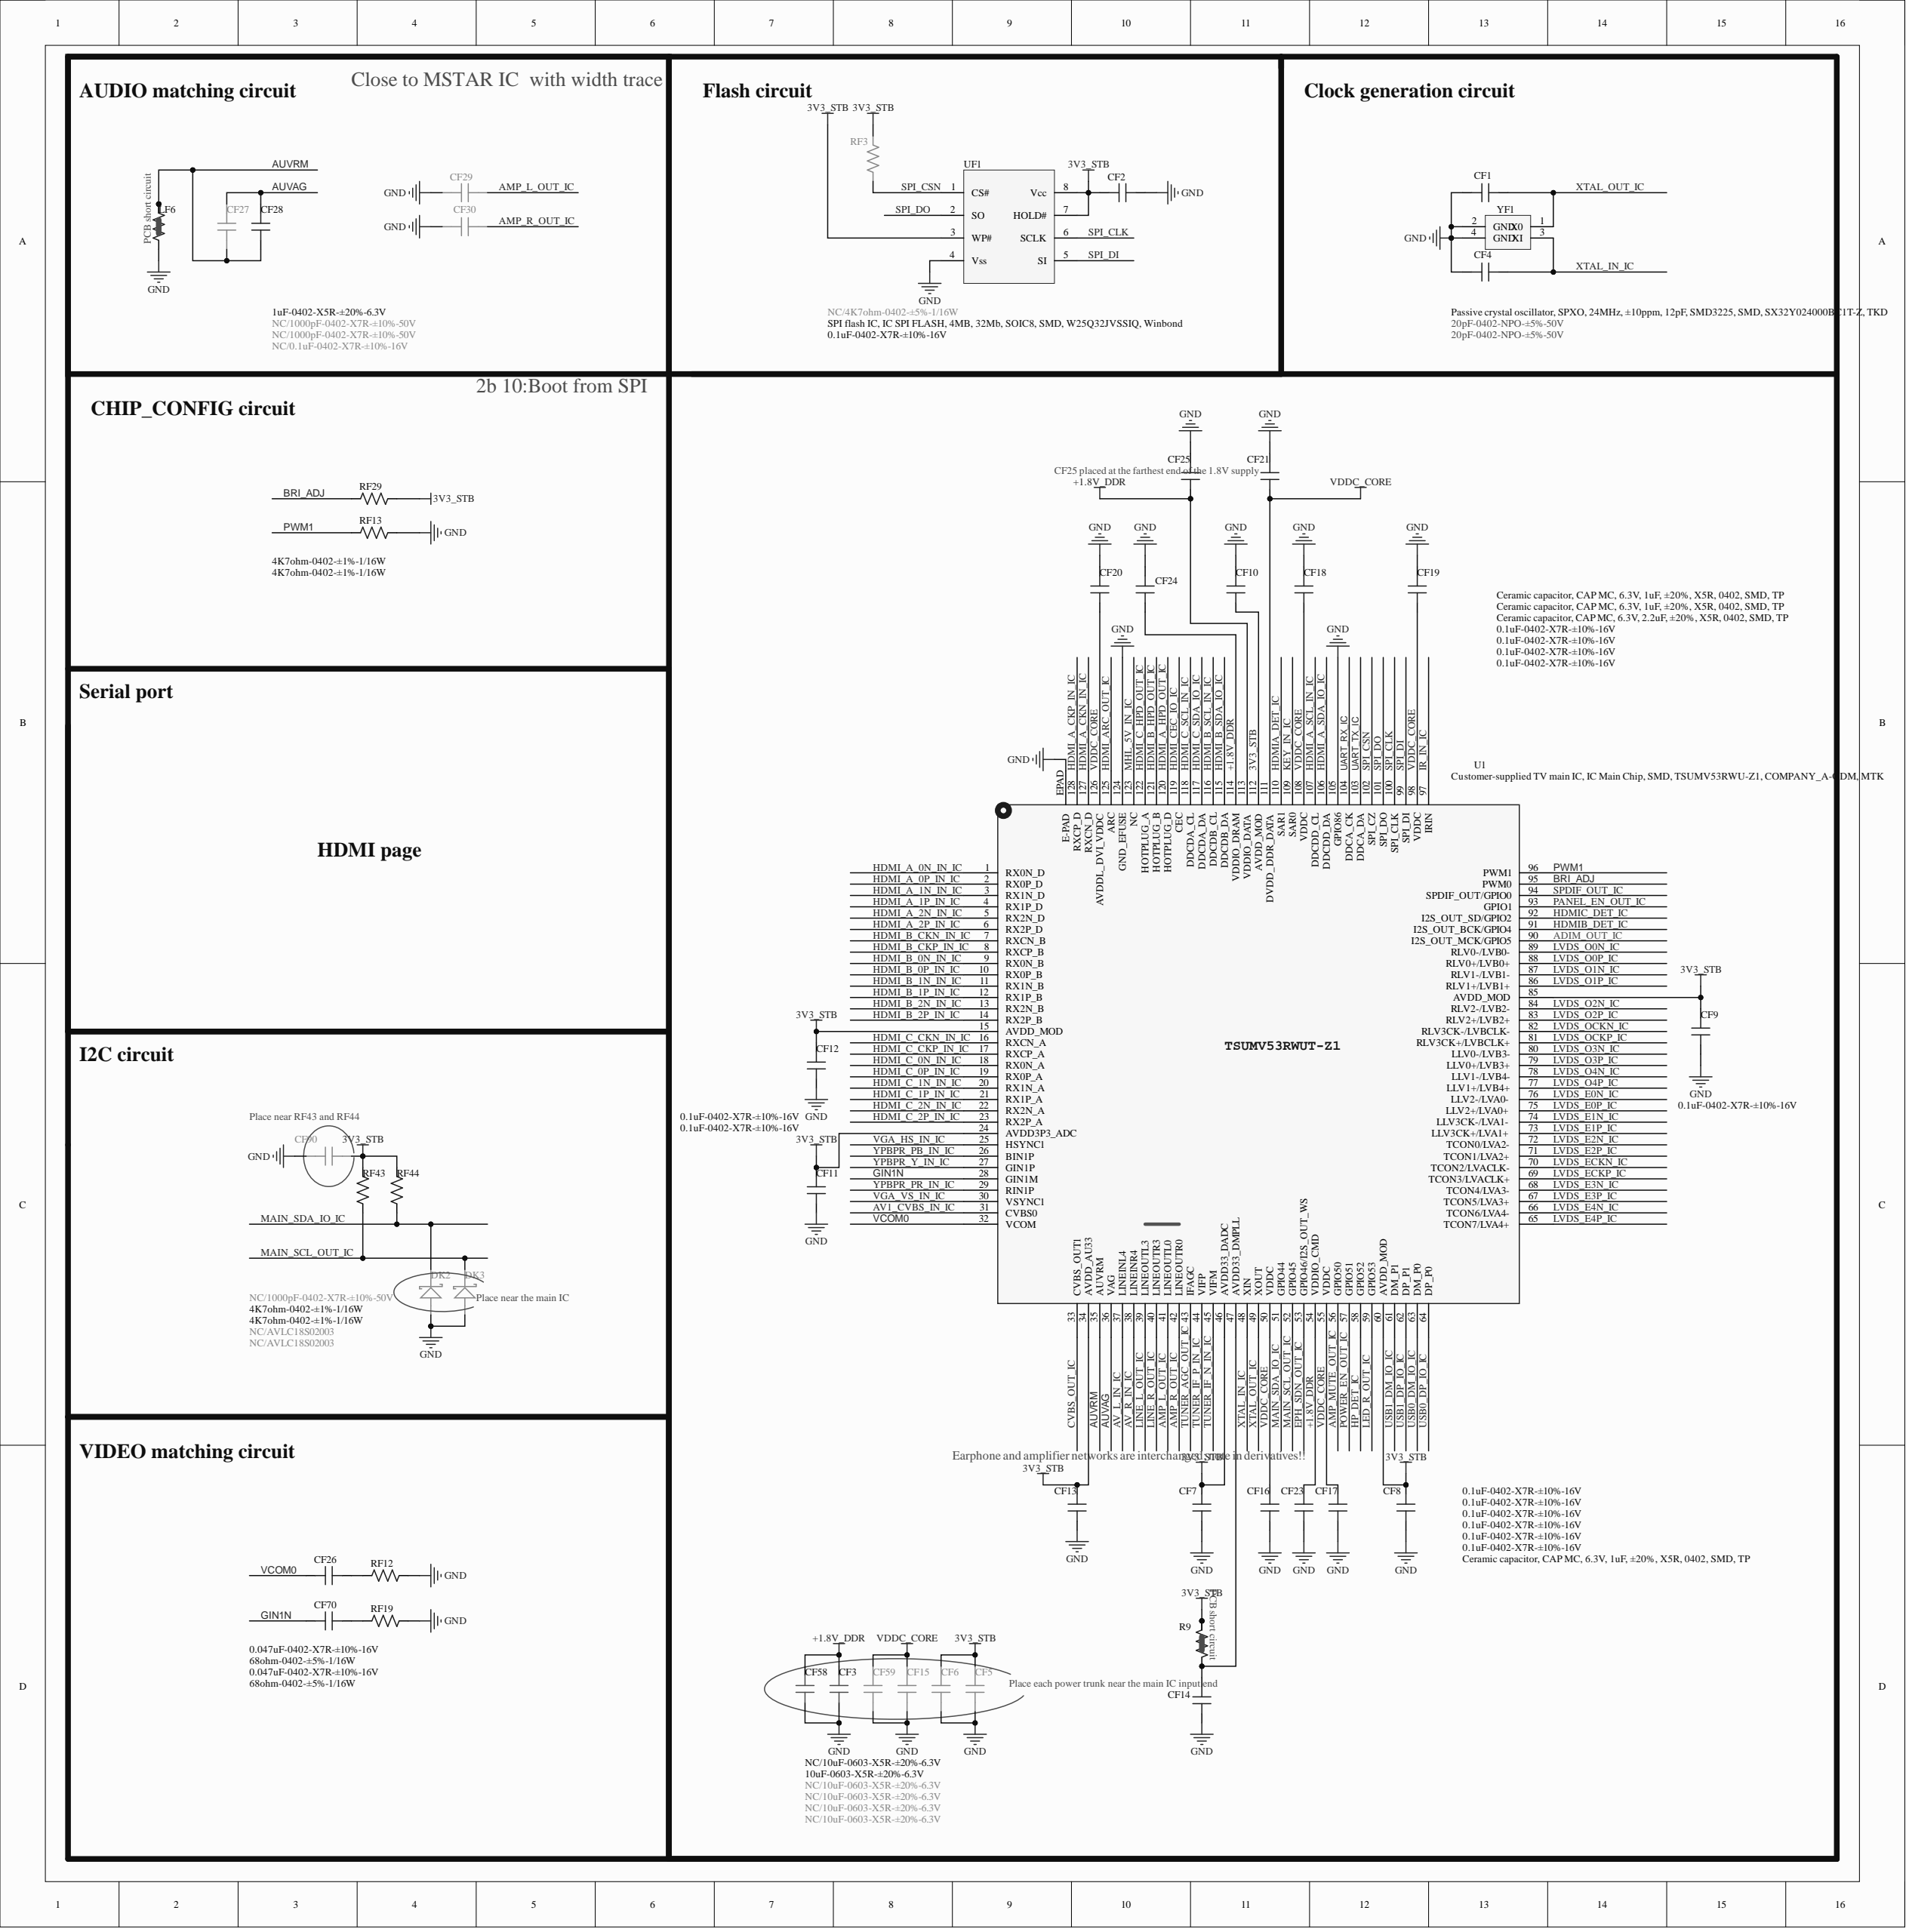Circuit board | Altium Designer | 541 parts | 263 nets | one sheet of the schematic
Parts on this sheet (reference | value | footprint):
CF1 | 20pF-0402-NPO-±5%-50V | C0402
CF2 | 0.1uF-0402-X7R-±10%-16V | C0402
CF3 | 10uF-0603-X5R-±20%-6.3V | C0603
CF4 | 20pF-0402-NPO-±5%-50V | C0402
CF5 | NC/10uF-0603-X5R-±20%-6.3V | C0603
CF6 | NC/10uF-0603-X5R-±20%-6.3V | C0603
CF7 | 0.1uF-0402-X7R-±10%-16V | C0402
CF8 | 0.1uF-0402-X7R-±10%-16V | C0402
CF9 | 0.1uF-0402-X7R-±10%-16V | C0402
CF10 | 0.1uF-0402-X7R-±10%-16V | C0402
CF11 | 0.1uF-0402-X7R-±10%-16V | C0402
CF12 | 0.1uF-0402-X7R-±10%-16V | C0402
CF13 | 0.1uF-0402-X7R-±10%-16V | C0402
CF14 | 0.1uF-0402-X7R-±10%-16V | C0402
CF15 | NC/10uF-0603-X5R-±20%-6.3V | C0603
CF16 | 0.1uF-0402-X7R-±10%-16V | C0402
CF17 | 0.1uF-0402-X7R-±10%-16V | C0402
CF18 | 0.1uF-0402-X7R-±10%-16V | C0402
CF19 | 0.1uF-0402-X7R-±10%-16V | C0402
CF20 | 0.1uF-0402-X7R-±10%-16V | C0402
CF21 | Ceramic capacitor, CAP MC, 6.3V, 1uF, ±20%, X5R, 0402, SMD, TP | C0402
CF23 | Ceramic capacitor, CAP MC, 6.3V, 1uF, ±20%, X5R, 0402, SMD, TP | C0402
CF24 | Ceramic capacitor, CAP MC, 6.3V, 1uF, ±20%, X5R, 0402, SMD, TP | C0402
CF25 | Ceramic capacitor, CAP MC, 6.3V, 2.2uF, ±20%, X5R, 0402, SMD, TP | C0402
CF26 | 0.047uF-0402-X7R-±10%-16V | C0402
CF27 | NC/0.1uF-0402-X7R-±10%-16V | C0402
CF28 | 1uF-0402-X5R-±20%-6.3V | C0402
CF29 | NC/1000pF-0402-X7R-±10%-50V | C0402
CF30 | NC/1000pF-0402-X7R-±10%-50V | C0402
CF58 | NC/10uF-0603-X5R-±20%-6.3V | C0603
CF59 | NC/10uF-0603-X5R-±20%-6.3V | C0603
CF70 | 0.047uF-0402-X7R-±10%-16V | C0402
CF90 | NC/1000pF-0402-X7R-±10%-50V | C0402
DK2 | NC/AVLC18S02003 | DIODE-S0402
DK3 | NC/AVLC18S02003 | DIODE-S0402
LF6 | NC/0ohm-0402-PCB | R0402SC
R9 | NC/0ohm-0402-PCB | R0402SC
RF3 | NC/4K7ohm-0402-±5%-1/16W | R0402
RF12 | 68ohm-0402-±5%-1/16W | R0402
RF13 | 4K7ohm-0402-±1%-1/16W | R0402
RF19 | 68ohm-0402-±5%-1/16W | R0402
RF29 | 4K7ohm-0402-±1%-1/16W | R0402
RF43 | 4K7ohm-0402-±1%-1/16W | R0402
RF44 | 4K7ohm-0402-±1%-1/16W | R0402
U1 | Customer-supplied TV main IC, IC Main Chip, SMD, TSUMV53RWU-Z1, COMPANY_A-ODM, MTK | QFN128/0.35-1
UF1 | SPI flash IC, IC SPI FLASH, 4MB, 32Mb, SOIC8, SMD, W25Q32JVSSIQ, Winbond | SOIC8
YF1 | Passive crystal oscillator, SPXO, 24MHz, ±10ppm, 12pF, SMD3225, SMD, SX32Y024000BC1T-Z, TKD | XTAL-S-3
Nets of these parts (net: part-pin ...):
YPBPR_Y_IN_IC: U1-27
YPBPR_PR_IN_IC: U1-29
YPBPR_PB_IN_IC: U1-26
XTAL_OUT_IC: CF1-2 YF1-1 U1-49
XTAL_IN_IC: CF4-2 YF1-3 U1-48
VDDC_CORE: CF15-2 CF16-2 CF17-2 CF18-1 CF19-1 CF20-2 CF21-1 CF59-2 U1-50 U1-55 U1-98 U1-108 U1-111 U1-126
VCOM0: CF26-1 U1-32
USB1_DP_IO_IC: U1-62
USB1_DM_IO_IC: U1-61
USB0_DP_IO_IC: U1-64
USB0_DM_IO_IC: U1-63
UART_TX_IC: U1-103
UART_RX_IC: U1-104
TUNER_IF_P_IN_IC: U1-44
TUNER_IF_N_IN_IC: U1-45
SPI_DO: UF1-2 U1-101
SPI_DI: UF1-5 U1-99
SPI_CSN: RF3-1 UF1-1 U1-102
SPI_CLK: UF1-6 U1-100
SPDIF_OUT_IC: U1-94
PWM1: RF13-1 U1-96
POWER_EN_OUT_IC: U1-57
PANEL_EN_OUT_IC: U1-93
NetCF70_2: CF70-2 RF19-1
NetCF26_2: CF26-2 RF12-1
NetCF14_2: CF14-2 R9-1 U1-47
MAIN_SDA_IO_IC: DK2-K RF44-2 U1-51
MAIN_SCL_OUT_IC: DK3-K RF43-2 U1-52
LVDS_OCKP_IC: U1-81
LVDS_OCKN_IC: U1-82
LVDS_O4P_IC: U1-77
LVDS_O4N_IC: U1-78
LVDS_O3P_IC: U1-79
LVDS_O3N_IC: U1-80
LVDS_O2P_IC: U1-83
LVDS_O2N_IC: U1-84
LVDS_O1P_IC: U1-86
LVDS_O1N_IC: U1-87
LVDS_O0P_IC: U1-88
LVDS_O0N_IC: U1-89
LVDS_ECKP_IC: U1-69
LVDS_ECKN_IC: U1-70
LVDS_E4P_IC: U1-65
LVDS_E4N_IC: U1-66
LVDS_E3P_IC: U1-67
LVDS_E3N_IC: U1-68
LVDS_E2P_IC: U1-71
LVDS_E2N_IC: U1-72
LVDS_E1P_IC: U1-73
LVDS_E1N_IC: U1-74
LVDS_E0P_IC: U1-75
LVDS_E0N_IC: U1-76
LINE_R_OUT_IC: U1-40
LINE_L_OUT_IC: U1-39
LED_R_OUT_IC: U1-59
KEY_IN_IC: U1-109
IR_IN_IC: U1-97
HP_DET_IC: U1-58
HDMIC_DET_IC: U1-92
HDMIB_DET_IC: U1-91
HDMIA_DET_IC: U1-110
HDMI_CEC_IO_IC: U1-119
HDMI_C_SDA_IO_IC: U1-117
HDMI_C_SCL_IN_IC: U1-118
HDMI_C_HPD_OUT_IC: U1-122
HDMI_C_CKP_IN_IC: U1-17
HDMI_C_CKN_IN_IC: U1-16
HDMI_C_2P_IN_IC: U1-23
HDMI_C_2N_IN_IC: U1-22
HDMI_C_1P_IN_IC: U1-21
HDMI_C_1N_IN_IC: U1-20
HDMI_C_0P_IN_IC: U1-19
HDMI_C_0N_IN_IC: U1-18
HDMI_B_SDA_IO_IC: U1-115
HDMI_B_SCL_IN_IC: U1-116
HDMI_B_HPD_OUT_IC: U1-121
HDMI_B_CKP_IN_IC: U1-8
HDMI_B_CKN_IN_IC: U1-7
HDMI_B_2P_IN_IC: U1-14
HDMI_B_2N_IN_IC: U1-13
HDMI_B_1P_IN_IC: U1-12
HDMI_B_1N_IN_IC: U1-11
HDMI_B_0P_IN_IC: U1-10
HDMI_B_0N_IN_IC: U1-9
HDMI_ARC_OUT_IC: U1-125
HDMI_A_SDA_IO_IC: U1-106
HDMI_A_SCL_IN_IC: U1-107
HDMI_A_HPD_OUT_IC: U1-120
HDMI_A_CKP_IN_IC: U1-128
HDMI_A_CKN_IN_IC: U1-127
HDMI_A_2P_IN_IC: U1-6
HDMI_A_2N_IN_IC: U1-5
HDMI_A_1P_IN_IC: U1-4
HDMI_A_1N_IN_IC: U1-3
HDMI_A_0P_IN_IC: U1-2
HDMI_A_0N_IN_IC: U1-1
GND: CF1-1 CF2-1 CF3-1 CF4-1 CF5-1 CF6-1 CF7-1 CF8-1 CF9-1 CF10-1 CF11-2 CF12-1 CF13-1 CF14-1 CF15-1 CF16-1 CF17-1 CF18-2 CF19-2 CF20-1 CF21-2 CF23-1 CF24-1 CF25-2 CF29-2 CF30-2 CF58-1 CF59-1 CF90-2 DK2-A DK3-A LF6-1 RF12-2 RF13-2 RF19-2 UF1-4 YF1-2 YF1-4 U1-105 U1-124 U1-EPAD
GIN1N: CF70-1 U1-28
EPH_SDN_OUT_IC: U1-53
BRI_ADJ: RF29-1 U1-95
AV_R_IN_IC: U1-38
AV_L_IN_IC: U1-37
AV1_CVBS_IN_IC: U1-31
AUVRM: CF27-1 CF28-1 LF6-2 LF6-3 U1-35
AUVAG: CF27-2 CF28-2 U1-36
AMP_R_OUT_IC: CF30-1 U1-42
AMP_MUTE_OUT_IC: U1-56
AMP_L_OUT_IC: CF29-1 U1-41
ADIM_OUT_IC: U1-90
+1.8V_DDR: CF3-2 CF23-2 CF24-2 CF25-1 CF58-2 U1-54 U1-113 U1-114
3V3_STB: CF2-2 CF5-2 CF6-2 CF7-2 CF8-2 CF9-2 CF10-2 CF11-1 CF12-2 CF13-2 CF90-1 R9-2 R9-3 RF3-2 RF29-2 RF43-1 RF44-1 UF1-3 UF1-7 UF1-8 U1-15 U1-24 U1-34 U1-46 U1-60 U1-85 U1-112